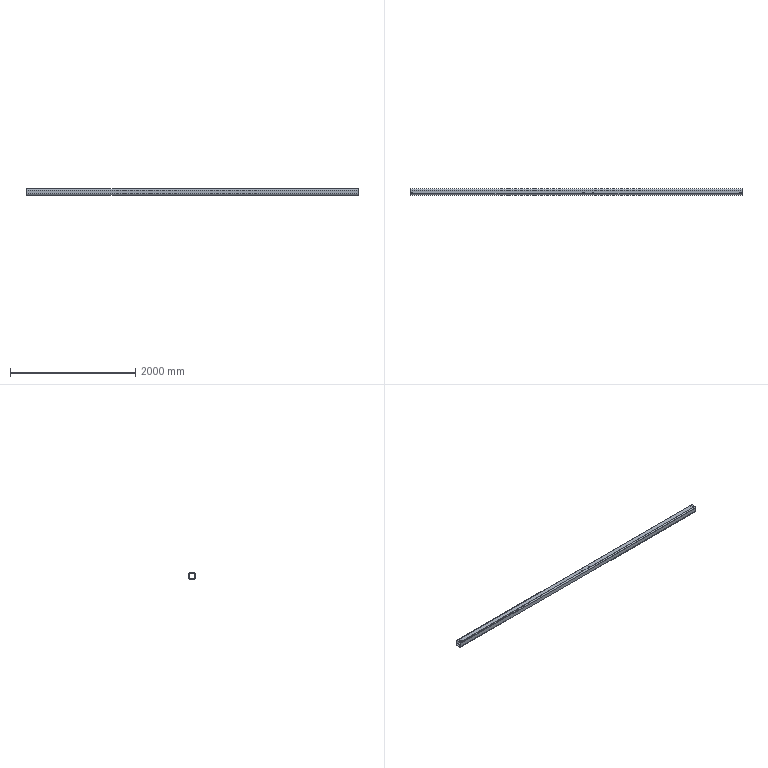Part | SolidWorks | features LPattern 3, ICE 1, RefAxis 1, WeldMemberFeat 1, WeldmentFeature 1 | 1 solid | 34 faces | box 5300 x 100 x 100 mm | volume 11061763 mm3 | cylinder 24 | plane 10 | commonest cylinder face diameters 22 x16 26.12 x4 38.12 x4